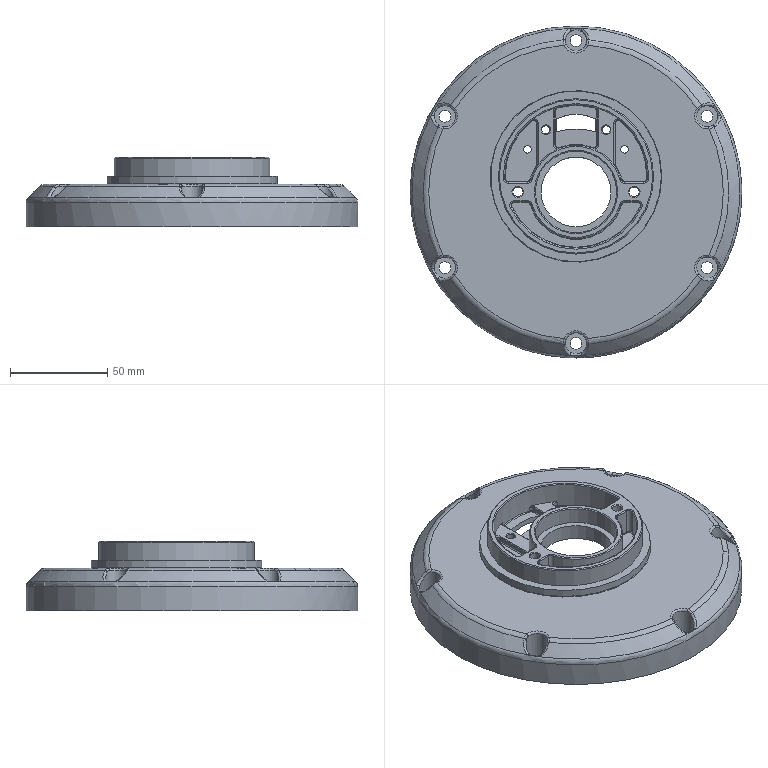NC program | NX | posted with a generic post | part box 171 x 171 x 36 mm
Lines 34957 to 35221 of 127321:
(点孔-A , TOOL : C8-L35)
N69894 T15 M6
N69896 G54
N69898 G17 G0 G90 X0. Y78. S1500 M3
N69900 G43 Z20. H15
N69902 G94 G81 G98 Z-33.5 F120. R-30.
N69904 X-67.55 Y39.
N69906 Y-39.
N69908 X0. Y-78.
N69910 X67.55 Y-39.
N69912 Y39.
N69914 G80
N69916 G0 X67.55 Y39. Z20.
(点孔-A_COPY_1 , TOOL : C8-L35)
N69918 X-15.5 Y32.
N69920 G81 Z-12.5 F120. R-9.
N69922 X15.5
N69924 G80
N69926 G0 X15.5 Y32. Z20.
(点孔-A_COPY_1_COPY_1 , TOOL : C8-L35)
N69928 X30. Y0.
N69930 G81 Z-1.5 F120. R2.
N69932 X-30.
N69934 X-25. Y22. Z-15.5 R-12.
N69936 X25.
N69938 G80
N69940 G0 X25. Y22. Z20.
N69942 M5
(点孔-A_COPY_1_COPY_1_COPY , TOOL : DK-3.5-L30)
N69944 T16 M6
N69946 G54
N69948 G17 G0 G90 X-25. Y22. S1200 M3
N69950 G43 Z20. H16
N69952 G94 G83 G98 Z-19.052 F70. Q2. R-12.
N69954 X25.
N69956 G80
N69958 G0 X25. Y22. Z20.
N69960 M5
(点孔-A_COPY_1_COPY , TOOL : DK-4.2-L35)
N69962 T17 M6
N69964 G54
N69966 G17 G0 G90 X-15.5 Y32. S1200 M3
N69968 G43 Z20. H17
N69970 G94 G83 G98 Z-19.262 F50. Q2. R-9.
N69972 X15.5
N69974 G80
N69976 G0 X15.5 Y32. Z20.
N69978 M5
(点孔-A_COPY , TOOL : DK-5.5-L40)
N69980 T18 M6
N69982 G54
N69984 G17 G0 G90 X0. Y78. S900 M3
N69986 G43 Z20. H18
N69988 G94 G83 G98 Z-38.652 F70. Q2. R-30.
N69990 X-67.55 Y39.
N69992 Y-39.
N69994 X0. Y-78.
N69996 X67.55 Y-39.
N69998 Y39.
N70000 G80
N70002 G0 X67.55 Y39. Z20.
N70004 M5
(点孔-A_COPY_COPY , TOOL : DK-5.0-L40)
N70006 T19 M6
N70008 G54
N70010 G17 G0 G90 X30. Y0. S900 M3
N70012 G43 Z20. H19
N70014 G94 G83 G98 Z-19.502 F70. Q2. R2.
N70016 X-30.
N70018 G80
N70020 G0 X-30. Y0. Z20.
N70022 M5
(点孔-A_COPY_1_COPY_1_COPY_1 , TOOL : C8-L35)
N70024 T15 M6
N70026 G54
N70028 G17 G0 G90 X-30. Y0. S2500 M3
N70030 G43 Z20. H15
N70032 G94 G81 G98 Z-2.8 F150. R2.
N70034 X30.
N70036 G80
N70038 G0 X30. Y0. Z20.
(点孔-A_COPY_1_COPY_1_COPY_1_COPY , TOOL : C8-L35)
N70040 X-15.5 Y32.
N70042 G81 Z-13.3 F150. R-9.
N70044 X15.5
N70046 G80
N70048 G0 X15.5 Y32. Z20.
(点孔-A_COPY_1_COPY_1_COPY_1_COPY_COPY , TOOL : C8-L35)
N70050 X-25. Y22.
N70052 G81 Z-16. F150. R-12.
N70054 X25.
N70056 G80
N70058 G0 X25. Y22. Z20.
(点孔-A_COPY_2 , TOOL : C8-L35)
N70060 X0. Y78.
N70062 G81 Z-35. F150. R-30.
N70064 X-67.55 Y39.
N70066 Y-39.
N70068 X0. Y-78.
N70070 X67.55 Y-39.
N70072 Y39.
N70074 G80
N70076 G0 X67.55 Y39. Z20.
N70078 M5
(铣孔-0.12 , TOOL : D4-L24)
N70080 T08 M6
N70082 G54
N70084 G17 G0 G90 X-67.55 Y39. S3500 M3
N70086 G43 Z20. H8
N70088 Z-31.5
N70090 G94 G3 X-67.11 Y38.56 R0.44 F1200.
N70092 X-66.67 Y39. R0.44
N70094 X-66.67 Y39. Z-31.85 I-0.88 J0.
N70096 X-66.67 Y39. Z-32.2 I-0.88 J0.
N70098 X-66.67 Y39. Z-32.55 I-0.88 J0.
N70100 X-66.67 Y39. Z-32.9 I-0.88 J0.
N70102 X-66.67 Y39. Z-33.25 I-0.88 J0.
N70104 X-66.67 Y39. Z-33.6 I-0.88 J0.
N70106 X-66.67 Y39. Z-33.95 I-0.88 J0.
N70108 X-66.67 Y39. Z-34.3 I-0.88 J0.
N70110 X-66.67 Y39. Z-34.65 I-0.88 J0.
N70112 X-66.67 Y39. Z-35. I-0.88 J0.
N70114 X-66.67 Y39. Z-35.35 I-0.88 J0.
N70116 X-66.67 Y39. Z-35.7 I-0.88 J0.
N70118 X-67.001 Y38.312 Z-36. R-0.88
N70120 X-67.001 Y38.312 R-0.88
N70122 X-66.717 Y38.715 R0.88
N70124 X-66.991 Y39.274 R0.44
N70126 X-67.55 Y39. R0.44
N70128 G0 Z20.
N70130 X0. Y78.
N70132 Z-31.5
N70134 G3 X0.44 Y77.56 R0.44
N70136 X0.88 Y78. R0.44
N70138 X0.88 Y78. Z-31.85 I-0.88 J0.
N70140 X0.88 Y78. Z-32.2 I-0.88 J0.
N70142 X0.88 Y78. Z-32.55 I-0.88 J0.
N70144 X0.88 Y78. Z-32.9 I-0.88 J0.
N70146 X0.88 Y78. Z-33.25 I-0.88 J0.
N70148 X0.88 Y78. Z-33.6 I-0.88 J0.
N70150 X0.88 Y78. Z-33.95 I-0.88 J0.
N70152 X0.88 Y78. Z-34.3 I-0.88 J0.
N70154 X0.88 Y78. Z-34.65 I-0.88 J0.
N70156 X0.88 Y78. Z-35. I-0.88 J0.
N70158 X0.88 Y78. Z-35.35 I-0.88 J0.
N70160 X0.88 Y78. Z-35.7 I-0.88 J0.
N70162 X0.549 Y77.312 Z-36. R-0.88
N70164 X0.549 Y77.312 R-0.88
N70166 X0.833 Y77.715 R0.88
N70168 X0.559 Y78.274 R0.44
N70170 X0. Y78. R0.44
N70172 G0 Z20.
N70174 X67.55 Y39.
N70176 Z-31.5
N70178 G3 X67.99 Y38.56 R0.44
N70180 X68.43 Y39. R0.44
N70182 X68.43 Y39. Z-31.85 I-0.88 J0.
N70184 X68.43 Y39. Z-32.2 I-0.88 J0.
N70186 X68.43 Y39. Z-32.55 I-0.88 J0.
N70188 X68.43 Y39. Z-32.9 I-0.88 J0.
N70190 X68.43 Y39. Z-33.25 I-0.88 J0.
N70192 X68.43 Y39. Z-33.6 I-0.88 J0.
N70194 X68.43 Y39. Z-33.95 I-0.88 J0.
N70196 X68.43 Y39. Z-34.3 I-0.88 J0.
N70198 X68.43 Y39. Z-34.65 I-0.88 J0.
N70200 X68.43 Y39. Z-35. I-0.88 J0.
N70202 X68.43 Y39. Z-35.35 I-0.88 J0.
N70204 X68.43 Y39. Z-35.7 I-0.88 J0.
N70206 X68.099 Y38.312 Z-36. R-0.88
N70208 X68.099 Y38.312 R-0.88
N70210 X68.383 Y38.715 R0.88
N70212 X68.109 Y39.274 R0.44
N70214 X67.55 Y39. R0.44
N70216 G0 Z20.
N70218 Y-39.
N70220 Z-31.5
N70222 G3 X67.99 Y-39.44 R0.44
N70224 X68.43 Y-39. R0.44
N70226 X68.43 Y-39. Z-31.85 I-0.88 J0.
N70228 X68.43 Y-39. Z-32.2 I-0.88 J0.
N70230 X68.43 Y-39. Z-32.55 I-0.88 J0.
N70232 X68.43 Y-39. Z-32.9 I-0.88 J0.
N70234 X68.43 Y-39. Z-33.25 I-0.88 J0.
N70236 X68.43 Y-39. Z-33.6 I-0.88 J0.
N70238 X68.43 Y-39. Z-33.95 I-0.88 J0.
N70240 X68.43 Y-39. Z-34.3 I-0.88 J0.
N70242 X68.43 Y-39. Z-34.65 I-0.88 J0.
N70244 X68.43 Y-39. Z-35. I-0.88 J0.
N70246 X68.43 Y-39. Z-35.35 I-0.88 J0.
N70248 X68.43 Y-39. Z-35.7 I-0.88 J0.
N70250 X68.099 Y-39.688 Z-36. R-0.88
N70252 X68.099 Y-39.688 R-0.88
N70254 X68.383 Y-39.285 R0.88
N70256 X68.109 Y-38.726 R0.44
N70258 X67.55 Y-39. R0.44
N70260 G0 Z20.
N70262 X0. Y-78.
N70264 Z-31.5
N70266 G3 X0.44 Y-78.44 R0.44
N70268 X0.88 Y-78. R0.44
N70270 X0.88 Y-78. Z-31.85 I-0.88 J0.
N70272 X0.88 Y-78. Z-32.2 I-0.88 J0.
N70274 X0.88 Y-78. Z-32.55 I-0.88 J0.
N70276 X0.88 Y-78. Z-32.9 I-0.88 J0.
N70278 X0.88 Y-78. Z-33.25 I-0.88 J0.
N70280 X0.88 Y-78. Z-33.6 I-0.88 J0.
N70282 X0.88 Y-78. Z-33.95 I-0.88 J0.
N70284 X0.88 Y-78. Z-34.3 I-0.88 J0.
N70286 X0.88 Y-78. Z-34.65 I-0.88 J0.
N70288 X0.88 Y-78. Z-35. I-0.88 J0.
N70290 X0.88 Y-78. Z-35.35 I-0.88 J0.
N70292 X0.88 Y-78. Z-35.7 I-0.88 J0.
N70294 X0.549 Y-78.688 Z-36. R-0.88
N70296 X0.549 Y-78.688 R-0.88
N70298 X0.833 Y-78.285 R0.88
N70300 X0.559 Y-77.726 R0.44
N70302 X0. Y-78. R0.44
N70304 G0 Z20.
N70306 X-67.55 Y-39.
N70308 Z-31.5
N70310 G3 X-67.11 Y-39.44 R0.44
N70312 X-66.67 Y-39. R0.44
N70314 X-66.67 Y-39. Z-31.85 I-0.88 J0.
N70316 X-66.67 Y-39. Z-32.2 I-0.88 J0.
N70318 X-66.67 Y-39. Z-32.55 I-0.88 J0.
N70320 X-66.67 Y-39. Z-32.9 I-0.88 J0.
N70322 X-66.67 Y-39. Z-33.25 I-0.88 J0.
N70324 X-66.67 Y-39. Z-33.6 I-0.88 J0.
N70326 X-66.67 Y-39. Z-33.95 I-0.88 J0.
N70328 X-66.67 Y-39. Z-34.3 I-0.88 J0.
N70330 X-66.67 Y-39. Z-34.65 I-0.88 J0.
N70332 X-66.67 Y-39. Z-35. I-0.88 J0.
N70334 X-66.67 Y-39. Z-35.35 I-0.88 J0.
N70336 X-66.67 Y-39. Z-35.7 I-0.88 J0.
N70338 X-67.001 Y-39.688 Z-36. R-0.88
N70340 X-67.001 Y-39.688 R-0.88
N70342 X-66.717 Y-39.285 R0.88
N70344 X-66.991 Y-38.726 R0.44
N70346 X-67.55 Y-39. R0.44
N70348 G0 Z20.
N70350 M5